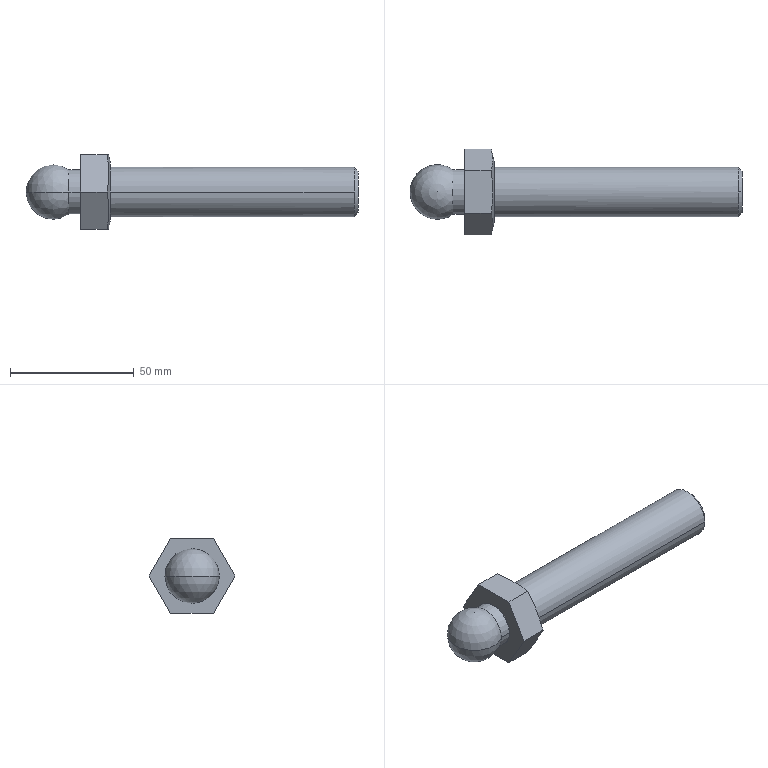Part | SolidWorks | features BaseBody 1 | 1 solid | 21 faces | box 134 x 34.641 x 30 mm | volume 46668 mm3 | plane 9 | cylinder 4 | cone 4 | torus 2 | sphere 2 | commonest cylinder face diameters 18 x2 20 x2
STEP:
#1=CARTESIAN_POINT('',(0.,-9.1,0.));
#2=VERTEX_POINT('',#1);
#3=CARTESIAN_POINT('',(0.,0.,-9.1));
#4=VERTEX_POINT('',#3);
#5=CARTESIAN_POINT('',(0.,-9.1,0.));
#6=CARTESIAN_POINT('',(0.,-9.1,-0.2784));
#7=CARTESIAN_POINT('',(0.,-9.081,-0.6942));
#8=CARTESIAN_POINT('',(0.,-9.026,-1.176));
#9=CARTESIAN_POINT('',(0.,-8.99,-1.416));
#10=CARTESIAN_POINT('',(0.,-8.972,-1.519));
#11=CARTESIAN_POINT('',(0.,-8.961,-1.587));
#12=CARTESIAN_POINT('',(0.,-8.955,-1.62));
#13=CARTESIAN_POINT('',(0.,-8.894,-1.946));
#14=CARTESIAN_POINT('',(0.,-8.793,-2.375));
#15=CARTESIAN_POINT('',(0.,-8.639,-2.866));
#16=CARTESIAN_POINT('',(0.,-8.553,-3.109));
#17=CARTESIAN_POINT('',(0.,-8.514,-3.212));
#18=CARTESIAN_POINT('',(0.,-8.488,-3.281));
#19=CARTESIAN_POINT('',(0.,-8.475,-3.314));
#20=CARTESIAN_POINT('',(0.,-8.348,-3.635));
#21=CARTESIAN_POINT('',(0.,-8.158,-4.054));
#22=CARTESIAN_POINT('',(0.,-7.899,-4.523));
#23=CARTESIAN_POINT('',(0.,-7.781,-4.72));
#24=CARTESIAN_POINT('',(0.,-7.7,-4.85));
#25=CARTESIAN_POINT('',(0.,-7.66,-4.914));
#26=CARTESIAN_POINT('',(0.,-7.273,-5.505));
#27=CARTESIAN_POINT('',(0.,-6.879,-5.991));
#28=CARTESIAN_POINT('',(0.,-6.213,-6.657));
#29=CARTESIAN_POINT('',(0.,-5.864,-6.971));
#30=CARTESIAN_POINT('',(0.,-5.431,-7.305));
#31=CARTESIAN_POINT('',(0.,-5.239,-7.441));
#32=CARTESIAN_POINT('',(0.,-5.11,-7.53));
#33=CARTESIAN_POINT('',(0.,-5.044,-7.575));
#34=CARTESIAN_POINT('',(0.,-4.722,-7.785));
#35=CARTESIAN_POINT('',(0.,-4.326,-8.017));
#36=CARTESIAN_POINT('',(0.,-3.844,-8.251));
#37=CARTESIAN_POINT('',(0.,-3.598,-8.359));
#38=CARTESIAN_POINT('',(0.,-3.492,-8.403));
#39=CARTESIAN_POINT('',(0.,-3.421,-8.433));
#40=CARTESIAN_POINT('',(0.,-3.384,-8.448));
#41=CARTESIAN_POINT('',(0.,-3.075,-8.57));
#42=CARTESIAN_POINT('',(0.,-2.658,-8.712));
#43=CARTESIAN_POINT('',(0.,-2.16,-8.842));
#44=CARTESIAN_POINT('',(0.,-1.909,-8.898));
#45=CARTESIAN_POINT('',(0.,-1.801,-8.92));
#46=CARTESIAN_POINT('',(0.,-1.728,-8.934));
#47=CARTESIAN_POINT('',(0.,-1.69,-8.942));
#48=CARTESIAN_POINT('',(0.,-1.109,-9.049));
#49=CARTESIAN_POINT('',(0.,-0.5571,-9.1));
#50=CARTESIAN_POINT('',(0.,0.,-9.1));
#51=B_SPLINE_CURVE_WITH_KNOTS('',3,(#5,#6,#7,#8,#9,#10,#11,#12,#13,#14,#15,#16,#17,#18,#19,#20,#21,#22,#23,#24,#25,#26,#27,#28,#29,#30,#31,#32,#33,#34,#35,#36,#37,#38,#39,#40,#41,#42,#43,#44,#45,#46,#47,#48,#49,#50),.UNSPECIFIED.,.F.,.F.,(4,1,1,1,2,2,1,1,1,2,2,1,1,2,2,2,1,1,2,2,1,1,1,2,2,1,1,1,2,2,4),(0.,0.0625,0.09375,0.1094,0.1172,0.125,0.1875,0.2188,0.2344,0.2422,0.25,0.3125,0.3438,0.3594,0.375,0.5,0.5625,0.5938,0.6094,0.625,0.6875,0.7188,0.7344,0.7422,0.75,0.8125,0.8438,0.8594,0.8672,0.875,1.),.UNSPECIFIED.);
#52=EDGE_CURVE('',#2,#4,#51,.T.);
#53=ORIENTED_EDGE('',*,*,#52,.F.);
#54=CARTESIAN_POINT('',(-0.1,-9.,0.));
#55=VERTEX_POINT('',#54);
#56=CARTESIAN_POINT('',(-0.1,-9.1,0.));
#57=DIRECTION('',(0.,0.,1.));
#58=DIRECTION('',(0.,-1.,0.));
#59=AXIS2_PLACEMENT_3D('',#56,#57,#58);
#60=CIRCLE('',#59,0.1);
#61=EDGE_CURVE('',#2,#55,#60,.T.);
#62=ORIENTED_EDGE('',*,*,#61,.T.);
#63=CARTESIAN_POINT('',(-0.1,9.,0.));
#64=VERTEX_POINT('',#63);
#65=CARTESIAN_POINT('',(-0.1,0.,0.));
#66=DIRECTION('',(-1.,0.,0.));
#67=DIRECTION('',(0.,0.,-1.));
#68=AXIS2_PLACEMENT_3D('',#65,#66,#67);
#69=CIRCLE('',#68,9.);
#70=EDGE_CURVE('',#64,#55,#69,.T.);
#71=ORIENTED_EDGE('',*,*,#70,.F.);
#72=CARTESIAN_POINT('',(0.,9.1,0.));
#73=VERTEX_POINT('',#72);
#74=CARTESIAN_POINT('',(-0.1,9.1,0.));
#75=DIRECTION('',(0.,0.,-1.));
#76=DIRECTION('',(-1.,0.,0.));
#77=AXIS2_PLACEMENT_3D('',#74,#75,#76);
#78=CIRCLE('',#77,0.1);
#79=EDGE_CURVE('',#73,#64,#78,.T.);
#80=ORIENTED_EDGE('',*,*,#79,.F.);
#81=CARTESIAN_POINT('',(0.,0.,-9.1));
#82=CARTESIAN_POINT('',(0.,0.2784,-9.1));
#83=CARTESIAN_POINT('',(0.,0.6942,-9.081));
#84=CARTESIAN_POINT('',(0.,1.176,-9.026));
#85=CARTESIAN_POINT('',(0.,1.416,-8.99));
#86=CARTESIAN_POINT('',(0.,1.519,-8.972));
#87=CARTESIAN_POINT('',(0.,1.587,-8.961));
#88=CARTESIAN_POINT('',(0.,1.62,-8.955));
#89=CARTESIAN_POINT('',(0.,1.946,-8.894));
#90=CARTESIAN_POINT('',(0.,2.375,-8.793));
#91=CARTESIAN_POINT('',(0.,2.866,-8.639));
#92=CARTESIAN_POINT('',(0.,3.109,-8.553));
#93=CARTESIAN_POINT('',(0.,3.212,-8.514));
#94=CARTESIAN_POINT('',(0.,3.281,-8.488));
#95=CARTESIAN_POINT('',(0.,3.314,-8.475));
#96=CARTESIAN_POINT('',(0.,3.635,-8.348));
#97=CARTESIAN_POINT('',(0.,4.054,-8.158));
#98=CARTESIAN_POINT('',(0.,4.523,-7.899));
#99=CARTESIAN_POINT('',(0.,4.72,-7.781));
#100=CARTESIAN_POINT('',(0.,4.85,-7.7));
#101=CARTESIAN_POINT('',(0.,4.914,-7.66));
#102=CARTESIAN_POINT('',(0.,5.505,-7.273));
#103=CARTESIAN_POINT('',(0.,5.991,-6.879));
#104=CARTESIAN_POINT('',(0.,6.657,-6.213));
#105=CARTESIAN_POINT('',(0.,6.971,-5.864));
#106=CARTESIAN_POINT('',(0.,7.305,-5.431));
#107=CARTESIAN_POINT('',(0.,7.441,-5.239));
#108=CARTESIAN_POINT('',(0.,7.53,-5.11));
#109=CARTESIAN_POINT('',(0.,7.575,-5.044));
#110=CARTESIAN_POINT('',(0.,7.785,-4.722));
#111=CARTESIAN_POINT('',(0.,8.017,-4.326));
#112=CARTESIAN_POINT('',(0.,8.251,-3.844));
#113=CARTESIAN_POINT('',(0.,8.359,-3.598));
#114=CARTESIAN_POINT('',(0.,8.403,-3.492));
#115=CARTESIAN_POINT('',(0.,8.433,-3.421));
#116=CARTESIAN_POINT('',(0.,8.448,-3.384));
#117=CARTESIAN_POINT('',(0.,8.57,-3.075));
#118=CARTESIAN_POINT('',(0.,8.712,-2.658));
#119=CARTESIAN_POINT('',(0.,8.842,-2.16));
#120=CARTESIAN_POINT('',(0.,8.898,-1.909));
#121=CARTESIAN_POINT('',(0.,8.92,-1.801));
#122=CARTESIAN_POINT('',(0.,8.934,-1.728));
#123=CARTESIAN_POINT('',(0.,8.942,-1.69));
#124=CARTESIAN_POINT('',(0.,9.049,-1.109));
#125=CARTESIAN_POINT('',(0.,9.1,-0.5562));
#126=CARTESIAN_POINT('',(0.,9.1,0.));
#127=B_SPLINE_CURVE_WITH_KNOTS('',3,(#81,#82,#83,#84,#85,#86,#87,#88,#89,#90,#91,#92,#93,#94,#95,#96,#97,#98,#99,#100,#101,#102,#103,#104,#105,#106,#107,#108,#109,#110,#111,#112,#113,#114,#115,#116,#117,#118,#119,#120,#121,#122,#123,#124,#125,#126),.UNSPECIFIED.,.F.,.F.,(4,1,1,1,2,2,1,1,1,2,2,1,1,2,2,2,1,1,2,2,1,1,1,2,2,1,1,1,2,2,4),(0.,0.03125,0.04687,0.05469,0.05859,0.0625,0.09375,0.1094,0.1172,0.1211,0.125,0.1562,0.1719,0.1797,0.1875,0.25,0.2812,0.2969,0.3047,0.3125,0.3437,0.3594,0.3672,0.3711,0.375,0.4062,0.4219,0.4297,0.4336,0.4375,0.5),.UNSPECIFIED.);
#128=EDGE_CURVE('',#4,#73,#127,.T.);
#129=ORIENTED_EDGE('',*,*,#128,.F.);
#130=EDGE_LOOP('',(#53,#62,#71,#80,#129));
#131=FACE_OUTER_BOUND('',#130,.T.);
#132=CARTESIAN_POINT('',(-0.1,0.,0.));
#133=DIRECTION('',(1.,0.,0.));
#134=DIRECTION('',(0.,1.,0.));
#135=AXIS2_PLACEMENT_3D('',#132,#133,#134);
#136=TOROIDAL_SURFACE('',#135,9.1,0.1);
#137=ADVANCED_FACE('',(#131),#136,.F.);
#138=CARTESIAN_POINT('',(-22.,0.,0.));
#139=VERTEX_POINT('',#138);
#140=CARTESIAN_POINT('',(-4.675,-9.,0.));
#141=VERTEX_POINT('',#140);
#142=CARTESIAN_POINT('',(-11.,0.,0.));
#143=DIRECTION('',(0.,0.,1.));
#144=DIRECTION('',(1.,0.,0.));
#145=AXIS2_PLACEMENT_3D('',#142,#143,#144);
#146=CIRCLE('',#145,11.);
#147=EDGE_CURVE('',#139,#141,#146,.T.);
#148=ORIENTED_EDGE('',*,*,#147,.F.);
#149=CARTESIAN_POINT('',(-4.675,9.,0.));
#150=VERTEX_POINT('',#149);
#151=CARTESIAN_POINT('',(-11.,0.,0.));
#152=DIRECTION('',(0.,0.,-1.));
#153=DIRECTION('',(-1.,0.,0.));
#154=AXIS2_PLACEMENT_3D('',#151,#152,#153);
#155=CIRCLE('',#154,11.);
#156=EDGE_CURVE('',#139,#150,#155,.T.);
#157=ORIENTED_EDGE('',*,*,#156,.T.);
#158=CARTESIAN_POINT('',(-4.675,0.,0.));
#159=DIRECTION('',(1.,0.,0.));
#160=DIRECTION('',(0.,-1.,0.));
#161=AXIS2_PLACEMENT_3D('',#158,#159,#160);
#162=CIRCLE('',#161,9.);
#163=EDGE_CURVE('',#141,#150,#162,.T.);
#164=ORIENTED_EDGE('',*,*,#163,.F.);
#165=EDGE_LOOP('',(#148,#157,#164));
#166=FACE_OUTER_BOUND('',#165,.T.);
#167=CARTESIAN_POINT('',(-11.,0.,0.));
#168=DIRECTION('',(0.,0.,-1.));
#169=DIRECTION('',(0.,-1.,0.));
#170=AXIS2_PLACEMENT_3D('',#167,#168,#169);
#171=SPHERICAL_SURFACE('',#170,11.);
#172=ADVANCED_FACE('',(#166),#171,.T.);
#173=CARTESIAN_POINT('',(110.466,0.,10.));
#174=VERTEX_POINT('',#173);
#175=CARTESIAN_POINT('',(110.466,10.,0.));
#176=VERTEX_POINT('',#175);
#177=CARTESIAN_POINT('',(110.466,0.,0.));
#178=DIRECTION('',(-1.,0.,0.));
#179=DIRECTION('',(0.,-1.,0.));
#180=AXIS2_PLACEMENT_3D('',#177,#178,#179);
#181=CIRCLE('',#180,10.);
#182=EDGE_CURVE('',#174,#176,#181,.T.);
#183=ORIENTED_EDGE('',*,*,#182,.T.);
#184=CARTESIAN_POINT('',(12.,10.,0.));
#185=VERTEX_POINT('',#184);
#186=CARTESIAN_POINT('',(61.233,10.,0.));
#187=DIRECTION('',(-1.,0.,0.));
#188=VECTOR('',#187,1000.);
#189=LINE('',#186,#188);
#190=EDGE_CURVE('',#176,#185,#189,.T.);
#191=ORIENTED_EDGE('',*,*,#190,.T.);
#192=CARTESIAN_POINT('',(12.,-10.,0.));
#193=VERTEX_POINT('',#192);
#194=CARTESIAN_POINT('',(12.,0.,0.));
#195=DIRECTION('',(1.,0.,0.));
#196=DIRECTION('',(0.,-1.,0.));
#197=AXIS2_PLACEMENT_3D('',#194,#195,#196);
#198=CIRCLE('',#197,10.);
#199=EDGE_CURVE('',#185,#193,#198,.T.);
#200=ORIENTED_EDGE('',*,*,#199,.T.);
#201=CARTESIAN_POINT('',(110.466,-10.,0.));
#202=VERTEX_POINT('',#201);
#203=CARTESIAN_POINT('',(61.233,-10.,0.));
#204=DIRECTION('',(-1.,0.,0.));
#205=VECTOR('',#204,1000.);
#206=LINE('',#203,#205);
#207=EDGE_CURVE('',#202,#193,#206,.T.);
#208=ORIENTED_EDGE('',*,*,#207,.F.);
#209=CARTESIAN_POINT('',(110.466,0.,0.));
#210=DIRECTION('',(-1.,0.,0.));
#211=DIRECTION('',(0.,-1.,0.));
#212=AXIS2_PLACEMENT_3D('',#209,#210,#211);
#213=CIRCLE('',#212,10.);
#214=EDGE_CURVE('',#202,#174,#213,.T.);
#215=ORIENTED_EDGE('',*,*,#214,.T.);
#216=EDGE_LOOP('',(#183,#191,#200,#208,#215));
#217=FACE_OUTER_BOUND('',#216,.T.);
#218=CARTESIAN_POINT('',(61.233,0.,0.));
#219=DIRECTION('',(-1.,0.,0.));
#220=DIRECTION('',(0.,-1.,0.));
#221=AXIS2_PLACEMENT_3D('',#218,#219,#220);
#222=CYLINDRICAL_SURFACE('',#221,10.);
#223=ADVANCED_FACE('',(#217),#222,.T.);
#224=CARTESIAN_POINT('',(112.,0.,8.466));
#225=VERTEX_POINT('',#224);
#226=CARTESIAN_POINT('',(112.,0.,-8.466));
#227=VERTEX_POINT('',#226);
#228=CARTESIAN_POINT('',(112.,0.,0.));
#229=DIRECTION('',(-1.,0.,0.));
#230=DIRECTION('',(0.,0.,1.));
#231=AXIS2_PLACEMENT_3D('',#228,#229,#230);
#232=CIRCLE('',#231,8.466);
#233=EDGE_CURVE('',#225,#227,#232,.T.);
#234=ORIENTED_EDGE('',*,*,#233,.T.);
#235=CARTESIAN_POINT('',(110.466,0.,-10.));
#236=VERTEX_POINT('',#235);
#237=CARTESIAN_POINT('',(110.466,0.,-10.));
#238=DIRECTION('',(-0.7071,0.,-0.7071));
#239=VECTOR('',#238,1000.);
#240=LINE('',#237,#239);
#241=EDGE_CURVE('',#227,#236,#240,.T.);
#242=ORIENTED_EDGE('',*,*,#241,.T.);
#243=CARTESIAN_POINT('',(110.466,0.,0.));
#244=DIRECTION('',(-1.,0.,0.));
#245=DIRECTION('',(0.,-1.,0.));
#246=AXIS2_PLACEMENT_3D('',#243,#244,#245);
#247=CIRCLE('',#246,10.);
#248=EDGE_CURVE('',#176,#236,#247,.T.);
#249=ORIENTED_EDGE('',*,*,#248,.F.);
#250=ORIENTED_EDGE('',*,*,#182,.F.);
#251=CARTESIAN_POINT('',(110.466,0.,10.));
#252=DIRECTION('',(-0.7071,0.,0.7071));
#253=VECTOR('',#252,1000.);
#254=LINE('',#251,#253);
#255=EDGE_CURVE('',#225,#174,#254,.T.);
#256=ORIENTED_EDGE('',*,*,#255,.F.);
#257=EDGE_LOOP('',(#234,#242,#249,#250,#256));
#258=FACE_OUTER_BOUND('',#257,.T.);
#259=CARTESIAN_POINT('',(110.466,0.,0.));
#260=DIRECTION('',(-1.,0.,0.));
#261=DIRECTION('',(0.,0.,1.));
#262=AXIS2_PLACEMENT_3D('',#259,#260,#261);
#263=CONICAL_SURFACE('',#262,10.,0.7854);
#264=ADVANCED_FACE('',(#258),#263,.T.);
#265=CARTESIAN_POINT('',(12.,12.,0.));
#266=VERTEX_POINT('',#265);
#267=CARTESIAN_POINT('',(12.,-12.,0.));
#268=VERTEX_POINT('',#267);
#269=CARTESIAN_POINT('',(12.,0.,0.));
#270=DIRECTION('',(1.,0.,0.));
#271=DIRECTION('',(0.,-1.,0.));
#272=AXIS2_PLACEMENT_3D('',#269,#270,#271);
#273=CIRCLE('',#272,12.);
#274=EDGE_CURVE('',#266,#268,#273,.T.);
#275=ORIENTED_EDGE('',*,*,#274,.F.);
#276=CARTESIAN_POINT('',(10.818,17.321,0.));
#277=VERTEX_POINT('',#276);
#278=CARTESIAN_POINT('',(10.811,17.352,0.));
#279=DIRECTION('',(-0.2169,0.9762,0.));
#280=VECTOR('',#279,1000.);
#281=LINE('',#278,#280);
#282=EDGE_CURVE('',#266,#277,#281,.T.);
#283=ORIENTED_EDGE('',*,*,#282,.T.);
#284=CARTESIAN_POINT('',(10.818,8.66,15.));
#285=VERTEX_POINT('',#284);
#286=CARTESIAN_POINT('',(10.818,17.321,0.));
#287=CARTESIAN_POINT('',(10.978,16.599,1.25));
#288=CARTESIAN_POINT('',(11.108,15.877,2.5));
#289=CARTESIAN_POINT('',(11.286,14.434,5.));
#290=CARTESIAN_POINT('',(11.38,12.99,7.5));
#291=CARTESIAN_POINT('',(11.286,11.547,10.));
#292=CARTESIAN_POINT('',(11.108,10.104,12.5));
#293=CARTESIAN_POINT('',(10.978,9.382,13.75));
#294=CARTESIAN_POINT('',(10.818,8.66,15.));
#295=B_SPLINE_CURVE_WITH_KNOTS('',3,(#286,#287,#288,#289,#290,#291,#292,#293,#294),.UNSPECIFIED.,.F.,.F.,(4,2,1,2,4),(0.,0.00433,0.00866,0.01299,0.01732),.UNSPECIFIED.);
#296=EDGE_CURVE('',#277,#285,#295,.T.);
#297=ORIENTED_EDGE('',*,*,#296,.T.);
#298=CARTESIAN_POINT('',(10.818,-8.66,15.));
#299=VERTEX_POINT('',#298);
#300=CARTESIAN_POINT('',(10.818,8.66,15.));
#301=CARTESIAN_POINT('',(10.978,7.217,15.));
#302=CARTESIAN_POINT('',(11.108,5.774,15.));
#303=CARTESIAN_POINT('',(11.286,2.887,15.));
#304=CARTESIAN_POINT('',(11.38,0.000000011,15.));
#305=CARTESIAN_POINT('',(11.286,-2.887,15.));
#306=CARTESIAN_POINT('',(11.108,-5.774,15.));
#307=CARTESIAN_POINT('',(10.978,-7.217,15.));
#308=CARTESIAN_POINT('',(10.818,-8.66,15.));
#309=B_SPLINE_CURVE_WITH_KNOTS('',3,(#300,#301,#302,#303,#304,#305,#306,#307,#308),.UNSPECIFIED.,.F.,.F.,(4,2,1,2,4),(0.,0.00433,0.00866,0.01299,0.01732),.UNSPECIFIED.);
#310=EDGE_CURVE('',#285,#299,#309,.T.);
#311=ORIENTED_EDGE('',*,*,#310,.T.);
#312=CARTESIAN_POINT('',(10.818,-17.321,0.));
#313=VERTEX_POINT('',#312);
#314=CARTESIAN_POINT('',(10.818,-8.66,15.));
#315=CARTESIAN_POINT('',(10.978,-9.382,13.75));
#316=CARTESIAN_POINT('',(11.108,-10.104,12.5));
#317=CARTESIAN_POINT('',(11.286,-11.547,10.));
#318=CARTESIAN_POINT('',(11.38,-12.99,7.5));
#319=CARTESIAN_POINT('',(11.286,-14.434,5.));
#320=CARTESIAN_POINT('',(11.108,-15.877,2.5));
#321=CARTESIAN_POINT('',(10.978,-16.599,1.25));
#322=CARTESIAN_POINT('',(10.818,-17.321,0.));
#323=B_SPLINE_CURVE_WITH_KNOTS('',3,(#314,#315,#316,#317,#318,#319,#320,#321,#322),.UNSPECIFIED.,.F.,.F.,(4,2,1,2,4),(0.,0.00433,0.00866,0.01299,0.01732),.UNSPECIFIED.);
#324=EDGE_CURVE('',#299,#313,#323,.T.);
#325=ORIENTED_EDGE('',*,*,#324,.T.);
#326=CARTESIAN_POINT('',(10.811,-17.352,0.));
#327=DIRECTION('',(-0.2169,-0.9762,0.));
#328=VECTOR('',#327,1000.);
#329=LINE('',#326,#328);
#330=EDGE_CURVE('',#268,#313,#329,.T.);
#331=ORIENTED_EDGE('',*,*,#330,.F.);
#332=EDGE_LOOP('',(#275,#283,#297,#311,#325,#331));
#333=FACE_OUTER_BOUND('',#332,.T.);
#334=CARTESIAN_POINT('',(10.811,0.,0.));
#335=DIRECTION('',(-1.,0.,0.));
#336=DIRECTION('',(0.,-1.,0.));
#337=AXIS2_PLACEMENT_3D('',#334,#335,#336);
#338=CONICAL_SURFACE('',#337,17.352,1.352);
#339=ADVANCED_FACE('',(#333),#338,.T.);
#340=CARTESIAN_POINT('',(-0.1,0.,0.));
#341=DIRECTION('',(-1.,0.,0.));
#342=DIRECTION('',(0.,0.,-1.));
#343=AXIS2_PLACEMENT_3D('',#340,#341,#342);
#344=CIRCLE('',#343,9.);
#345=EDGE_CURVE('',#55,#64,#344,.T.);
#346=ORIENTED_EDGE('',*,*,#345,.T.);
#347=CARTESIAN_POINT('',(-2.388,9.,0.));
#348=DIRECTION('',(-1.,0.,0.));
#349=VECTOR('',#348,1000.);
#350=LINE('',#347,#349);
#351=EDGE_CURVE('',#64,#150,#350,.T.);
#352=ORIENTED_EDGE('',*,*,#351,.T.);
#353=CARTESIAN_POINT('',(-4.675,0.,0.));
#354=DIRECTION('',(1.,0.,0.));
#355=DIRECTION('',(0.,-1.,0.));
#356=AXIS2_PLACEMENT_3D('',#353,#354,#355);
#357=CIRCLE('',#356,9.);
#358=EDGE_CURVE('',#150,#141,#357,.T.);
#359=ORIENTED_EDGE('',*,*,#358,.T.);
#360=CARTESIAN_POINT('',(-2.388,-9.,0.));
#361=DIRECTION('',(-1.,0.,0.));
#362=VECTOR('',#361,1000.);
#363=LINE('',#360,#362);
#364=EDGE_CURVE('',#55,#141,#363,.T.);
#365=ORIENTED_EDGE('',*,*,#364,.F.);
#366=EDGE_LOOP('',(#346,#352,#359,#365));
#367=FACE_OUTER_BOUND('',#366,.T.);
#368=CARTESIAN_POINT('',(-2.388,0.,0.));
#369=DIRECTION('',(-1.,0.,0.));
#370=DIRECTION('',(0.,-1.,0.));
#371=AXIS2_PLACEMENT_3D('',#368,#369,#370);
#372=CYLINDRICAL_SURFACE('',#371,9.);
#373=ADVANCED_FACE('',(#367),#372,.T.);
#374=ORIENTED_EDGE('',*,*,#128,.T.);
#375=CARTESIAN_POINT('',(0.,0.,9.1));
#376=VERTEX_POINT('',#375);
#377=CARTESIAN_POINT('',(0.,9.1,0.));
#378=CARTESIAN_POINT('',(0.,9.1,0.2781));
#379=CARTESIAN_POINT('',(0.,9.081,0.6937));
#380=CARTESIAN_POINT('',(0.,9.026,1.176));
#381=CARTESIAN_POINT('',(0.,8.99,1.416));
#382=CARTESIAN_POINT('',(0.,8.972,1.519));
#383=CARTESIAN_POINT('',(0.,8.961,1.587));
#384=CARTESIAN_POINT('',(0.,8.955,1.62));
#385=CARTESIAN_POINT('',(0.,8.894,1.946));
#386=CARTESIAN_POINT('',(0.,8.793,2.375));
#387=CARTESIAN_POINT('',(0.,8.639,2.866));
#388=CARTESIAN_POINT('',(0.,8.553,3.109));
#389=CARTESIAN_POINT('',(0.,8.514,3.212));
#390=CARTESIAN_POINT('',(0.,8.488,3.281));
#391=CARTESIAN_POINT('',(0.,8.475,3.314));
#392=CARTESIAN_POINT('',(0.,8.348,3.635));
#393=CARTESIAN_POINT('',(0.,8.158,4.054));
#394=CARTESIAN_POINT('',(0.,7.899,4.523));
#395=CARTESIAN_POINT('',(0.,7.781,4.72));
#396=CARTESIAN_POINT('',(0.,7.7,4.85));
#397=CARTESIAN_POINT('',(0.,7.66,4.914));
#398=CARTESIAN_POINT('',(0.,7.273,5.505));
#399=CARTESIAN_POINT('',(0.,6.879,5.991));
#400=CARTESIAN_POINT('',(0.,6.213,6.657));
#401=CARTESIAN_POINT('',(0.,5.864,6.971));
#402=CARTESIAN_POINT('',(0.,5.431,7.305));
#403=CARTESIAN_POINT('',(0.,5.239,7.441));
#404=CARTESIAN_POINT('',(0.,5.11,7.53));
#405=CARTESIAN_POINT('',(0.,5.044,7.575));
#406=CARTESIAN_POINT('',(0.,4.722,7.785));
#407=CARTESIAN_POINT('',(0.,4.326,8.017));
#408=CARTESIAN_POINT('',(0.,3.844,8.251));
#409=CARTESIAN_POINT('',(0.,3.598,8.359));
#410=CARTESIAN_POINT('',(0.,3.492,8.403));
#411=CARTESIAN_POINT('',(0.,3.421,8.433));
#412=CARTESIAN_POINT('',(0.,3.384,8.448));
#413=CARTESIAN_POINT('',(0.,3.075,8.57));
#414=CARTESIAN_POINT('',(0.,2.658,8.712));
#415=CARTESIAN_POINT('',(0.,2.16,8.842));
#416=CARTESIAN_POINT('',(0.,1.909,8.898));
#417=CARTESIAN_POINT('',(0.,1.801,8.92));
#418=CARTESIAN_POINT('',(0.,1.728,8.934));
#419=CARTESIAN_POINT('',(0.,1.69,8.942));
#420=CARTESIAN_POINT('',(0.,1.109,9.049));
#421=CARTESIAN_POINT('',(0.,0.5571,9.1));
#422=CARTESIAN_POINT('',(0.,0.,9.1));
#423=B_SPLINE_CURVE_WITH_KNOTS('',3,(#377,#378,#379,#380,#381,#382,#383,#384,#385,#386,#387,#388,#389,#390,#391,#392,#393,#394,#395,#396,#397,#398,#399,#400,#401,#402,#403,#404,#405,#406,#407,#408,#409,#410,#411,#412,#413,#414,#415,#416,#417,#418,#419,#420,#421,#422),.UNSPECIFIED.,.F.,.F.,(4,1,1,1,2,2,1,1,1,2,2,1,1,2,2,2,1,1,2,2,1,1,1,2,2,1,1,1,2,2,4),(0.5,0.5312,0.5469,0.5547,0.5586,0.5625,0.5937,0.6094,0.6172,0.6211,0.625,0.6562,0.6719,0.6797,0.6875,0.75,0.7812,0.7969,0.8047,0.8125,0.8437,0.8594,0.8672,0.8711,0.875,0.9062,0.9219,0.9297,0.9336,0.9375,1.),.UNSPECIFIED.);
#424=EDGE_CURVE('',#73,#376,#423,.T.);
#425=ORIENTED_EDGE('',*,*,#424,.T.);
#426=CARTESIAN_POINT('',(0.,0.,9.1));
#427=CARTESIAN_POINT('',(0.,-0.2784,9.1));
#428=CARTESIAN_POINT('',(0.,-0.6942,9.081));
#429=CARTESIAN_POINT('',(0.,-1.176,9.026));
#430=CARTESIAN_POINT('',(0.,-1.416,8.99));
#431=CARTESIAN_POINT('',(0.,-1.519,8.972));
#432=CARTESIAN_POINT('',(0.,-1.587,8.961));
#433=CARTESIAN_POINT('',(0.,-1.62,8.955));
#434=CARTESIAN_POINT('',(0.,-1.946,8.894));
#435=CARTESIAN_POINT('',(0.,-2.375,8.793));
#436=CARTESIAN_POINT('',(0.,-2.866,8.639));
#437=CARTESIAN_POINT('',(0.,-3.109,8.553));
#438=CARTESIAN_POINT('',(0.,-3.212,8.514));
#439=CARTESIAN_POINT('',(0.,-3.281,8.488));
#440=CARTESIAN_POINT('',(0.,-3.314,8.475));
#441=CARTESIAN_POINT('',(0.,-3.635,8.348));
#442=CARTESIAN_POINT('',(0.,-4.054,8.158));
#443=CARTESIAN_POINT('',(0.,-4.523,7.899));
#444=CARTESIAN_POINT('',(0.,-4.72,7.781));
#445=CARTESIAN_POINT('',(0.,-4.85,7.7));
#446=CARTESIAN_POINT('',(0.,-4.914,7.66));
#447=CARTESIAN_POINT('',(0.,-5.505,7.273));
#448=CARTESIAN_POINT('',(0.,-5.991,6.879));
#449=CARTESIAN_POINT('',(0.,-6.657,6.213));
#450=CARTESIAN_POINT('',(0.,-6.971,5.864));
#451=CARTESIAN_POINT('',(0.,-7.305,5.431));
#452=CARTESIAN_POINT('',(0.,-7.441,5.239));
#453=CARTESIAN_POINT('',(0.,-7.53,5.11));
#454=CARTESIAN_POINT('',(0.,-7.575,5.044));
#455=CARTESIAN_POINT('',(0.,-7.785,4.722));
#456=CARTESIAN_POINT('',(0.,-8.017,4.326));
#457=CARTESIAN_POINT('',(0.,-8.251,3.844));
#458=CARTESIAN_POINT('',(0.,-8.359,3.598));
#459=CARTESIAN_POINT('',(0.,-8.403,3.492));
#460=CARTESIAN_POINT('',(0.,-8.433,3.421));
#461=CARTESIAN_POINT('',(0.,-8.448,3.384));
#462=CARTESIAN_POINT('',(0.,-8.57,3.075));
#463=CARTESIAN_POINT('',(0.,-8.712,2.658));
#464=CARTESIAN_POINT('',(0.,-8.842,2.16));
#465=CARTESIAN_POINT('',(0.,-8.898,1.909));
#466=CARTESIAN_POINT('',(0.,-8.92,1.801));
#467=CARTESIAN_POINT('',(0.,-8.934,1.728));
#468=CARTESIAN_POINT('',(0.,-8.942,1.69));
#469=CARTESIAN_POINT('',(0.,-9.049,1.109));
#470=CARTESIAN_POINT('',(0.,-9.1,0.5571));
#471=CARTESIAN_POINT('',(0.,-9.1,0.));
#472=B_SPLINE_CURVE_WITH_KNOTS('',3,(#426,#427,#428,#429,#430,#431,#432,#433,#434,#435,#436,#437,#438,#439,#440,#441,#442,#443,#444,#445,#446,#447,#448,#449,#450,#451,#452,#453,#454,#455,#456,#457,#458,#459,#460,#461,#462,#463,#464,#465,#466,#467,#468,#469,#470,#471),.UNSPECIFIED.,.F.,.F.,(4,1,1,1,2,2,1,1,1,2,2,1,1,2,2,2,1,1,2,2,1,1,1,2,2,1,1,1,2,2,4),(0.,0.0625,0.09375,0.1094,0.1172,0.125,0.1875,0.2187,0.2344,0.2422,0.25,0.3125,0.3437,0.3594,0.375,0.5,0.5625,0.5938,0.6094,0.625,0.6875,0.7188,0.7344,0.7422,0.75,0.8125,0.8438,0.8594,0.8672,0.875,1.),.UNSPECIFIED.);
#473=EDGE_CURVE('',#376,#2,#472,.T.);
#474=ORIENTED_EDGE('',*,*,#473,.T.);
#475=ORIENTED_EDGE('',*,*,#52,.T.);
#476=EDGE_LOOP('',(#374,#425,#474,#475));
#477=FACE_BOUND('',#476,.T.);
#478=CARTESIAN_POINT('',(0.,-8.66,-15.));
#479=VERTEX_POINT('',#478);
#480=CARTESIAN_POINT('',(0.,-17.321,0.));
#481=VERTEX_POINT('',#480);
#482=CARTESIAN_POINT('',(0.,-17.321,0.));
#483=DIRECTION('',(0.,-0.5,0.866));
#484=VECTOR('',#483,1000.);
#485=LINE('',#482,#484);
#486=EDGE_CURVE('',#479,#481,#485,.T.);
#487=ORIENTED_EDGE('',*,*,#486,.T.);
#488=CARTESIAN_POINT('',(0.,-8.66,15.));
#489=VERTEX_POINT('',#488);
#490=CARTESIAN_POINT('',(0.,-8.66,15.));
#491=DIRECTION('',(0.,0.5,0.866));
#492=VECTOR('',#491,1000.);
#493=LINE('',#490,#492);
#494=EDGE_CURVE('',#481,#489,#493,.T.);
#495=ORIENTED_EDGE('',*,*,#494,.T.);
#496=CARTESIAN_POINT('',(0.,8.66,15.));
#497=VERTEX_POINT('',#496);
#498=CARTESIAN_POINT('',(0.,8.66,15.));
#499=DIRECTION('',(0.,1.,0.));
#500=VECTOR('',#499,1000.);
#501=LINE('',#498,#500);
#502=EDGE_CURVE('',#489,#497,#501,.T.);
#503=ORIENTED_EDGE('',*,*,#502,.T.);
#504=CARTESIAN_POINT('',(0.,17.321,0.));
#505=VERTEX_POINT('',#504);
#506=CARTESIAN_POINT('',(0.,17.321,0.));
#507=DIRECTION('',(0.,0.5,-0.866));
#508=VECTOR('',#507,1000.);
#509=LINE('',#506,#508);
#510=EDGE_CURVE('',#497,#505,#509,.T.);
#511=ORIENTED_EDGE('',*,*,#510,.T.);
#512=CARTESIAN_POINT('',(0.,8.66,-15.));
#513=VERTEX_POINT('',#512);
#514=CARTESIAN_POINT('',(0.,8.66,-15.));
#515=DIRECTION('',(0.,-0.5,-0.866));
#516=VECTOR('',#515,1000.);
#517=LINE('',#514,#516);
#518=EDGE_CURVE('',#505,#513,#517,.T.);
#519=ORIENTED_EDGE('',*,*,#518,.T.);
#520=CARTESIAN_POINT('',(0.,-8.66,-15.));
#521=DIRECTION('',(0.,-1.,0.));
#522=VECTOR('',#521,1000.);
#523=LINE('',#520,#522);
#524=EDGE_CURVE('',#513,#479,#523,.T.);
#525=ORIENTED_EDGE('',*,*,#524,.T.);
#526=EDGE_LOOP('',(#487,#495,#503,#511,#519,#525));
#527=FACE_OUTER_BOUND('',#526,.T.);
#528=CARTESIAN_POINT('',(0.,-13.925,0.));
#529=DIRECTION('',(-1.,0.,0.));
#530=DIRECTION('',(0.,1.,0.));
#531=AXIS2_PLACEMENT_3D('',#528,#529,#530);
#532=PLANE('',#531);
#533=ADVANCED_FACE('',(#477,#527),#532,.T.);
#534=CARTESIAN_POINT('',(0.,-17.321,0.));
#535=DIRECTION('',(-1.,0.,0.));
#536=VECTOR('',#535,1000.);
#537=LINE('',#534,#536);
#538=EDGE_CURVE('',#313,#481,#537,.T.);
#539=ORIENTED_EDGE('',*,*,#538,.T.);
#540=ORIENTED_EDGE('',*,*,#486,.F.);
#541=CARTESIAN_POINT('',(10.818,-8.66,-15.));
#542=VERTEX_POINT('',#541);
#543=CARTESIAN_POINT('',(0.,-8.66,-15.));
#544=DIRECTION('',(1.,0.,0.));
#545=VECTOR('',#544,1000.);
#546=LINE('',#543,#545);
#547=EDGE_CURVE('',#479,#542,#546,.T.);
#548=ORIENTED_EDGE('',*,*,#547,.T.);
#549=CARTESIAN_POINT('',(10.818,-17.321,0.));
#550=CARTESIAN_POINT('',(10.978,-16.599,-1.25));
#551=CARTESIAN_POINT('',(11.108,-15.877,-2.5));
#552=CARTESIAN_POINT('',(11.286,-14.434,-5.));
#553=CARTESIAN_POINT('',(11.38,-12.99,-7.5));
#554=CARTESIAN_POINT('',(11.286,-11.547,-10.));
#555=CARTESIAN_POINT('',(11.108,-10.104,-12.5));
#556=CARTESIAN_POINT('',(10.978,-9.382,-13.75));
#557=CARTESIAN_POINT('',(10.818,-8.66,-15.));
#558=B_SPLINE_CURVE_WITH_KNOTS('',3,(#549,#550,#551,#552,#553,#554,#555,#556,#557),.UNSPECIFIED.,.F.,.F.,(4,2,1,2,4),(0.,0.00433,0.00866,0.01299,0.01732),.UNSPECIFIED.);
#559=EDGE_CURVE('',#313,#542,#558,.T.);
#560=ORIENTED_EDGE('',*,*,#559,.F.);
#561=EDGE_LOOP('',(#539,#540,#548,#560));
#562=FACE_OUTER_BOUND('',#561,.T.);
#563=CARTESIAN_POINT('',(0.,-17.321,0.));
#564=DIRECTION('',(0.,0.866,0.5));
#565=DIRECTION('',(1.,0.,0.));
#566=AXIS2_PLACEMENT_3D('',#563,#564,#565);
#567=PLANE('',#566);
#568=ADVANCED_FACE('',(#562),#567,.F.);
#569=ORIENTED_EDGE('',*,*,#547,.F.);
#570=ORIENTED_EDGE('',*,*,#524,.F.);
#571=CARTESIAN_POINT('',(10.818,8.66,-15.));
#572=VERTEX_POINT('',#571);
#573=CARTESIAN_POINT('',(0.,8.66,-15.));
#574=DIRECTION('',(1.,0.,0.));
#575=VECTOR('',#574,1000.);
#576=LINE('',#573,#575);
#577=EDGE_CURVE('',#513,#572,#576,.T.);
#578=ORIENTED_EDGE('',*,*,#577,.T.);
#579=CARTESIAN_POINT('',(10.818,-8.66,-15.));
#580=CARTESIAN_POINT('',(10.978,-7.217,-15.));
#581=CARTESIAN_POINT('',(11.108,-5.774,-15.));
#582=CARTESIAN_POINT('',(11.286,-2.887,-15.));
#583=CARTESIAN_POINT('',(11.38,-0.000000011,-15.));
#584=CARTESIAN_POINT('',(11.286,2.887,-15.));
#585=CARTESIAN_POINT('',(11.108,5.774,-15.));
#586=CARTESIAN_POINT('',(10.978,7.217,-15.));
#587=CARTESIAN_POINT('',(10.818,8.66,-15.));
#588=B_SPLINE_CURVE_WITH_KNOTS('',3,(#579,#580,#581,#582,#583,#584,#585,#586,#587),.UNSPECIFIED.,.F.,.F.,(4,2,1,2,4),(0.,0.00433,0.00866,0.01299,0.01732),.UNSPECIFIED.);
#589=EDGE_CURVE('',#542,#572,#588,.T.);
#590=ORIENTED_EDGE('',*,*,#589,.F.);
#591=EDGE_LOOP('',(#569,#570,#578,#590));
#592=FACE_OUTER_BOUND('',#591,.T.);
#593=CARTESIAN_POINT('',(0.,-8.66,-15.));
#594=DIRECTION('',(0.,0.,1.));
#595=DIRECTION('',(1.,0.,0.));
#596=AXIS2_PLACEMENT_3D('',#593,#594,#595);
#597=PLANE('',#596);
#598=ADVANCED_FACE('',(#592),#597,.F.);
#599=ORIENTED_EDGE('',*,*,#577,.F.);
#600=ORIENTED_EDGE('',*,*,#518,.F.);
#601=CARTESIAN_POINT('',(0.,17.321,0.));
#602=DIRECTION('',(1.,0.,0.));
#603=VECTOR('',#602,1000.);
#604=LINE('',#601,#603);
#605=EDGE_CURVE('',#505,#277,#604,.T.);
#606=ORIENTED_EDGE('',*,*,#605,.T.);
#607=CARTESIAN_POINT('',(10.818,8.66,-15.));
#608=CARTESIAN_POINT('',(10.978,9.382,-13.75));
#609=CARTESIAN_POINT('',(11.108,10.104,-12.5));
#610=CARTESIAN_POINT('',(11.286,11.547,-10.));
#611=CARTESIAN_POINT('',(11.38,12.99,-7.5));
#612=CARTESIAN_POINT('',(11.286,14.434,-5.));
#613=CARTESIAN_POINT('',(11.108,15.877,-2.5));
#614=CARTESIAN_POINT('',(10.978,16.599,-1.25));
#615=CARTESIAN_POINT('',(10.818,17.321,0.));
#616=B_SPLINE_CURVE_WITH_KNOTS('',3,(#607,#608,#609,#610,#611,#612,#613,#614,#615),.UNSPECIFIED.,.F.,.F.,(4,2,1,2,4),(0.,0.00433,0.00866,0.01299,0.01732),.UNSPECIFIED.);
#617=EDGE_CURVE('',#572,#277,#616,.T.);
#618=ORIENTED_EDGE('',*,*,#617,.F.);
#619=EDGE_LOOP('',(#599,#600,#606,#618));
#620=FACE_OUTER_BOUND('',#619,.T.);
#621=CARTESIAN_POINT('',(0.,8.66,-15.));
#622=DIRECTION('',(0.,-0.866,0.5));
#623=DIRECTION('',(-1.,0.,0.));
#624=AXIS2_PLACEMENT_3D('',#621,#622,#623);
#625=PLANE('',#624);
#626=ADVANCED_FACE('',(#620),#625,.F.);
#627=ORIENTED_EDGE('',*,*,#605,.F.);
#628=ORIENTED_EDGE('',*,*,#510,.F.);
#629=CARTESIAN_POINT('',(0.,8.66,15.));
#630=DIRECTION('',(1.,0.,0.));
#631=VECTOR('',#630,1000.);
#632=LINE('',#629,#631);
#633=EDGE_CURVE('',#497,#285,#632,.T.);
#634=ORIENTED_EDGE('',*,*,#633,.T.);
#635=ORIENTED_EDGE('',*,*,#296,.F.);
#636=EDGE_LOOP('',(#627,#628,#634,#635));
#637=FACE_OUTER_BOUND('',#636,.T.);
#638=CARTESIAN_POINT('',(0.,17.321,0.));
#639=DIRECTION('',(0.,-0.866,-0.5));
#640=DIRECTION('',(0.,0.5,-0.866));
#641=AXIS2_PLACEMENT_3D('',#638,#639,#640);
#642=PLANE('',#641);
#643=ADVANCED_FACE('',(#637),#642,.F.);
#644=ORIENTED_EDGE('',*,*,#633,.F.);
#645=ORIENTED_EDGE('',*,*,#502,.F.);
#646=CARTESIAN_POINT('',(0.,-8.66,15.));
#647=DIRECTION('',(1.,0.,0.));
#648=VECTOR('',#647,1000.);
#649=LINE('',#646,#648);
#650=EDGE_CURVE('',#489,#299,#649,.T.);
#651=ORIENTED_EDGE('',*,*,#650,.T.);
#652=ORIENTED_EDGE('',*,*,#310,.F.);
#653=EDGE_LOOP('',(#644,#645,#651,#652));
#654=FACE_OUTER_BOUND('',#653,.T.);
#655=CARTESIAN_POINT('',(0.,8.66,15.));
#656=DIRECTION('',(0.,0.,-1.));
#657=DIRECTION('',(0.,-1.,0.));
#658=AXIS2_PLACEMENT_3D('',#655,#656,#657);
#659=PLANE('',#658);
#660=ADVANCED_FACE('',(#654),#659,.F.);
#661=ORIENTED_EDGE('',*,*,#650,.F.);
#662=ORIENTED_EDGE('',*,*,#494,.F.);
#663=ORIENTED_EDGE('',*,*,#538,.F.);
#664=ORIENTED_EDGE('',*,*,#324,.F.);
#665=EDGE_LOOP('',(#661,#662,#663,#664));
#666=FACE_OUTER_BOUND('',#665,.T.);
#667=CARTESIAN_POINT('',(0.,-8.66,15.));
#668=DIRECTION('',(0.,0.866,-0.5));
#669=DIRECTION('',(-1.,0.,0.));
#670=AXIS2_PLACEMENT_3D('',#667,#668,#669);
#671=PLANE('',#670);
#672=ADVANCED_FACE('',(#666),#671,.F.);
#673=ORIENTED_EDGE('',*,*,#233,.F.);
#674=CARTESIAN_POINT('',(112.,0.,0.));
#675=DIRECTION('',(-1.,0.,0.));
#676=DIRECTION('',(0.,0.,1.));
#677=AXIS2_PLACEMENT_3D('',#674,#675,#676);
#678=CIRCLE('',#677,8.466);
#679=EDGE_CURVE('',#227,#225,#678,.T.);
#680=ORIENTED_EDGE('',*,*,#679,.F.);
#681=EDGE_LOOP('',(#673,#680));
#682=FACE_OUTER_BOUND('',#681,.T.);
#683=CARTESIAN_POINT('',(112.,-4.233,0.));
#684=DIRECTION('',(1.,0.,0.));
#685=DIRECTION('',(0.,0.,-1.));
#686=AXIS2_PLACEMENT_3D('',#683,#684,#685);
#687=PLANE('',#686);
#688=ADVANCED_FACE('',(#682),#687,.T.);
#689=CARTESIAN_POINT('',(12.,0.,0.));
#690=DIRECTION('',(1.,0.,0.));
#691=DIRECTION('',(0.,-1.,0.));
#692=AXIS2_PLACEMENT_3D('',#689,#690,#691);
#693=CIRCLE('',#692,10.);
#694=EDGE_CURVE('',#193,#185,#693,.T.);
#695=ORIENTED_EDGE('',*,*,#694,.F.);
#696=ORIENTED_EDGE('',*,*,#199,.F.);
#697=EDGE_LOOP('',(#695,#696));
#698=FACE_BOUND('',#697,.T.);
#699=CARTESIAN_POINT('',(12.,0.,0.));
#700=DIRECTION('',(1.,0.,0.));
#701=DIRECTION('',(0.,-1.,0.));
#702=AXIS2_PLACEMENT_3D('',#699,#700,#701);
#703=CIRCLE('',#702,12.);
#704=EDGE_CURVE('',#268,#266,#703,.T.);
#705=ORIENTED_EDGE('',*,*,#704,.T.);
#706=ORIENTED_EDGE('',*,*,#274,.T.);
#707=EDGE_LOOP('',(#705,#706));
#708=FACE_OUTER_BOUND('',#707,.T.);
#709=CARTESIAN_POINT('',(12.,-11.,0.));
#710=DIRECTION('',(1.,0.,0.));
#711=DIRECTION('',(0.,1.,0.));
#712=AXIS2_PLACEMENT_3D('',#709,#710,#711);
#713=PLANE('',#712);
#714=ADVANCED_FACE('',(#698,#708),#713,.T.);
#715=ORIENTED_EDGE('',*,*,#351,.F.);
#716=ORIENTED_EDGE('',*,*,#70,.T.);
#717=ORIENTED_EDGE('',*,*,#364,.T.);
#718=ORIENTED_EDGE('',*,*,#163,.T.);
#719=EDGE_LOOP('',(#715,#716,#717,#718));
#720=FACE_OUTER_BOUND('',#719,.T.);
#721=CARTESIAN_POINT('',(-2.388,0.,0.));
#722=DIRECTION('',(-1.,0.,0.));
#723=DIRECTION('',(0.,-1.,0.));
#724=AXIS2_PLACEMENT_3D('',#721,#722,#723);
#725=CYLINDRICAL_SURFACE('',#724,9.);
#726=ADVANCED_FACE('',(#720),#725,.T.);
#727=ORIENTED_EDGE('',*,*,#282,.F.);
#728=ORIENTED_EDGE('',*,*,#704,.F.);
#729=ORIENTED_EDGE('',*,*,#330,.T.);
#730=ORIENTED_EDGE('',*,*,#559,.T.);
#731=ORIENTED_EDGE('',*,*,#589,.T.);
#732=ORIENTED_EDGE('',*,*,#617,.T.);
#733=EDGE_LOOP('',(#727,#728,#729,#730,#731,#732));
#734=FACE_OUTER_BOUND('',#733,.T.);
#735=CARTESIAN_POINT('',(10.811,0.,0.));
#736=DIRECTION('',(-1.,0.,0.));
#737=DIRECTION('',(0.,-1.,0.));
#738=AXIS2_PLACEMENT_3D('',#735,#736,#737);
#739=CONICAL_SURFACE('',#738,17.352,1.352);
#740=ADVANCED_FACE('',(#734),#739,.T.);
#741=ORIENTED_EDGE('',*,*,#241,.F.);
#742=ORIENTED_EDGE('',*,*,#679,.T.);
#743=ORIENTED_EDGE('',*,*,#255,.T.);
#744=ORIENTED_EDGE('',*,*,#214,.F.);
#745=CARTESIAN_POINT('',(110.466,0.,0.));
#746=DIRECTION('',(-1.,0.,0.));
#747=DIRECTION('',(0.,-1.,0.));
#748=AXIS2_PLACEMENT_3D('',#745,#746,#747);
#749=CIRCLE('',#748,10.);
#750=EDGE_CURVE('',#236,#202,#749,.T.);
#751=ORIENTED_EDGE('',*,*,#750,.F.);
#752=EDGE_LOOP('',(#741,#742,#743,#744,#751));
#753=FACE_OUTER_BOUND('',#752,.T.);
#754=CARTESIAN_POINT('',(110.466,0.,0.));
#755=DIRECTION('',(-1.,0.,0.));
#756=DIRECTION('',(0.,0.,1.));
#757=AXIS2_PLACEMENT_3D('',#754,#755,#756);
#758=CONICAL_SURFACE('',#757,10.,0.7854);
#759=ADVANCED_FACE('',(#753),#758,.T.);
#760=ORIENTED_EDGE('',*,*,#190,.F.);
#761=ORIENTED_EDGE('',*,*,#248,.T.);
#762=ORIENTED_EDGE('',*,*,#750,.T.);
#763=ORIENTED_EDGE('',*,*,#207,.T.);
#764=ORIENTED_EDGE('',*,*,#694,.T.);
#765=EDGE_LOOP('',(#760,#761,#762,#763,#764));
#766=FACE_OUTER_BOUND('',#765,.T.);
#767=CARTESIAN_POINT('',(61.233,0.,0.));
#768=DIRECTION('',(-1.,0.,0.));
#769=DIRECTION('',(0.,-1.,0.));
#770=AXIS2_PLACEMENT_3D('',#767,#768,#769);
#771=CYLINDRICAL_SURFACE('',#770,10.);
#772=ADVANCED_FACE('',(#766),#771,.T.);
#773=ORIENTED_EDGE('',*,*,#156,.F.);
#774=ORIENTED_EDGE('',*,*,#147,.T.);
#775=ORIENTED_EDGE('',*,*,#358,.F.);
#776=EDGE_LOOP('',(#773,#774,#775));
#777=FACE_OUTER_BOUND('',#776,.T.);
#778=CARTESIAN_POINT('',(-11.,0.,0.));
#779=DIRECTION('',(0.,0.,-1.));
#780=DIRECTION('',(0.,-1.,0.));
#781=AXIS2_PLACEMENT_3D('',#778,#779,#780);
#782=SPHERICAL_SURFACE('',#781,11.);
#783=ADVANCED_FACE('',(#777),#782,.T.);
#784=ORIENTED_EDGE('',*,*,#61,.F.);
#785=ORIENTED_EDGE('',*,*,#473,.F.);
#786=ORIENTED_EDGE('',*,*,#424,.F.);
#787=ORIENTED_EDGE('',*,*,#79,.T.);
#788=ORIENTED_EDGE('',*,*,#345,.F.);
#789=EDGE_LOOP('',(#784,#785,#786,#787,#788));
#790=FACE_OUTER_BOUND('',#789,.T.);
#791=CARTESIAN_POINT('',(-0.1,0.,0.));
#792=DIRECTION('',(1.,0.,0.));
#793=DIRECTION('',(0.,1.,0.));
#794=AXIS2_PLACEMENT_3D('',#791,#792,#793);
#795=TOROIDAL_SURFACE('',#794,9.1,0.1);
#796=ADVANCED_FACE('',(#790),#795,.F.);
#797=CLOSED_SHELL('',(#137,#172,#223,#264,#339,#373,#533,#568,#598,#626,#643,#660,#672,#688,#714,#726,#740,#759,#772,#783,#796));
#798=MANIFOLD_SOLID_BREP('',#797);
#799=CARTESIAN_POINT('',(0.,0.,0.));
#800=DIRECTION('',(0.,0.,1.));
#801=DIRECTION('',(1.,0.,0.));
#802=AXIS2_PLACEMENT_3D('',#799,#800,#801);
#803=(LENGTH_UNIT()NAMED_UNIT(*)SI_UNIT(.MILLI.,.METRE.));
#804=UNCERTAINTY_MEASURE_WITH_UNIT(LENGTH_MEASURE(0.00001),#803,'','');
#805=(NAMED_UNIT(*)PLANE_ANGLE_UNIT()SI_UNIT($,.RADIAN.));
#806=(NAMED_UNIT(*)SI_UNIT($,.STERADIAN.)SOLID_ANGLE_UNIT());
#807=(GEOMETRIC_REPRESENTATION_CONTEXT(3)GLOBAL_UNCERTAINTY_ASSIGNED_CONTEXT((#804))GLOBAL_UNIT_ASSIGNED_CONTEXT((#803,#805,#806))REPRESENTATION_CONTEXT('',''));
#808=ADVANCED_BREP_SHAPE_REPRESENTATION('',(#798,#802),#807);